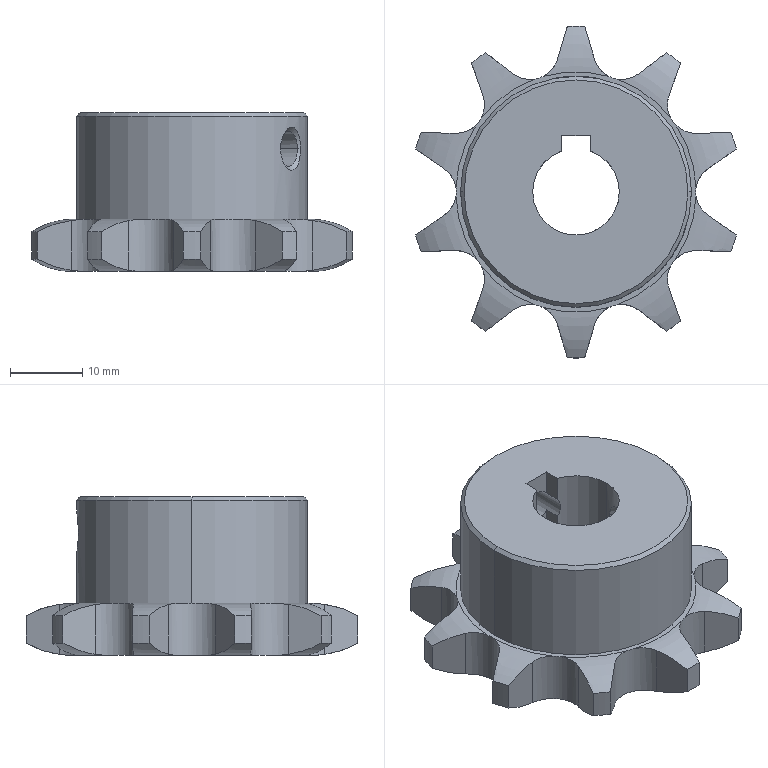Part | NX | features BREP 1 | 1 solid | 87 faces | box 44.433 x 46 x 22 mm | volume 17001 mm3 | cylinder 32 | plane 29 | torus 20 | cone 6 | commonest cylinder face diameters 7.92 x13 46 x10 4.917 x4 12 x3 32 x2